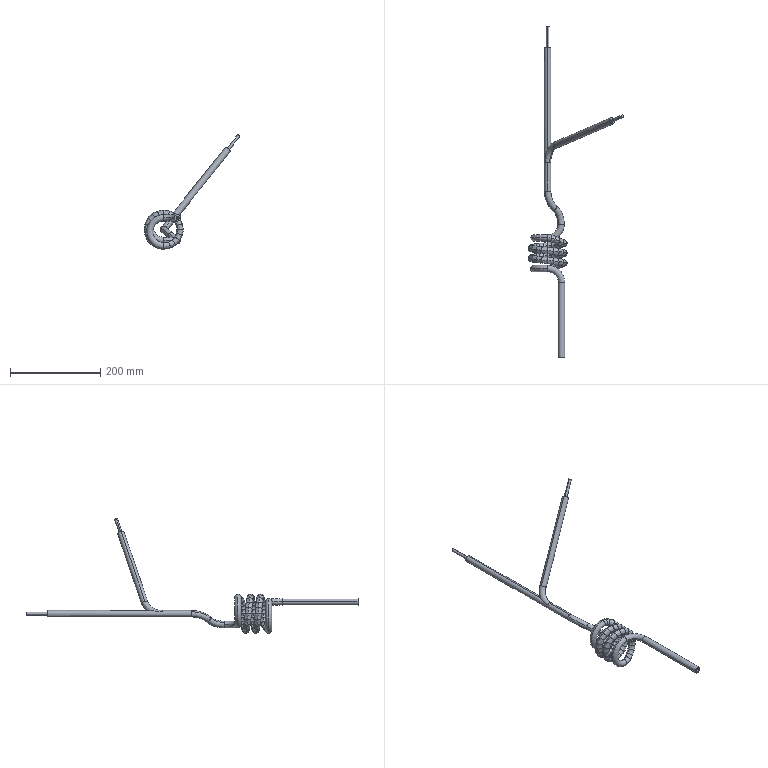Part | NX | features BREP 2 | 2 solids | 254 faces | box 212.038 x 735.189 x 253.179 mm | volume 227004 mm3 | spline 204 | torus 27 | cylinder 16 | plane 7 | commonest cylinder face diameters 6.35 x8 14.3 x6 3.91 x2